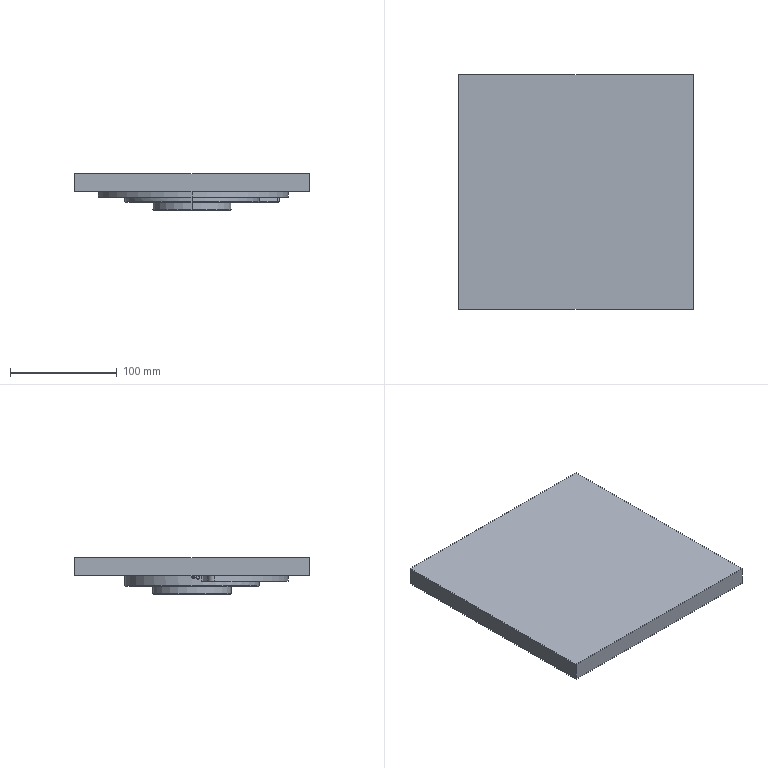NC program | NX | posted with a generic post | part box 220 x 220 x 34.5 mm
Lines 75 to 964 of 14163:
(ADAPTIVE_MILLING , TOOL : D10)
N118 T03 M6
N120 G54
N122 G17 G0 G90 X95.263 Y20.832 S8000 M3
N124 G43 Z30. H3
N126 Z-14.
N128 G94 G1 Z-17. F1000.
N130 X93.186 Y20.519 F3500.
N132 G3 X92.826 Y20.05 R0.517
N134 X93.039 Y13.768 R32.792
N136 G2 X93.561 Y-8.186 R106.889
N138 X-81.594 Y-46.533 R93.929
N140 X-84.05 Y-44.249 R11.158
N142 G3 X-84.843 Y-44.271 R0.524
N144 G1 X-86.022 Y-45.738
N146 G3 X-85.392 Y-46.489 R0.523
N148 G1 Z-14.
N150 G0 Z30.
N152 X95.262 Y18.312
N154 Z-14.
N156 G1 Z-17. F1000.
N158 G3 X94.965 Y19.276 R0.505 F3500.
N160 G1 X93.056 Y18.777
N162 G3 X92.762 Y18.381 R0.516
N164 X92.304 Y12.752 R16.402
N166 G2 X92.863 Y-0.982 R181.125
N168 X-79.677 Y-47.733 R92.885
N170 G1 X-79.748 Y-47.63
N172 X-79.823 Y-47.53
N174 X-79.915 Y-47.445
N176 X-79.934 Y-47.43
N178 G2 X-81.619 Y-46.513 R12.102
N180 G3 X-82.433 Y-46.766 R0.523
N182 G1 X-82.979 Y-48.467
N184 G3 X-82.283 Y-49.037 R0.523
N186 G1 Z-14.
N188 G0 Z30.
N190 X94.895 Y16.439
N192 Z-14.
N194 G1 Z-17. F1000.
N196 G3 X94.676 Y17.416 R0.505 F3500.
N198 G1 X92.8 Y17.246
N200 G3 X92.43 Y16.866 R0.513
N202 G2 X91.946 Y15.492 R15.396
N204 G3 X91.567 Y10.898 R17.162
N206 G2 X91.808 Y-1.348 R262.213
N208 X-77.715 Y-48.908 R91.827
N210 G3 X-78.616 Y-47.86 R3.744
N212 G2 X-80.011 Y-47.39 R8.929
N214 G3 X-80.769 Y-47.81 R0.523
N216 G1 X-80.913 Y-49.545
N218 G3 X-80.21 Y-49.992 R0.524
N220 G1 Z-14.
N222 G0 Z30.
N224 X94.546 Y15.319
N226 Z-14.
N228 G1 Z-17. F1000.
N230 G3 X94.362 Y16.297 R0.505 F3500.
N232 G1 X92.484 Y16.265
N234 G3 X92.109 Y15.965 R0.516
N236 X91.136 Y13.442 R15.341
N238 X90.756 Y7.716 R26.833
N240 G2 X90.504 Y-6.776 R155.471
N242 X-75.608 Y-50.206 R90.761
N244 G3 X-77.263 Y-48.18 R10.711
N246 X-78.032 Y-48.035 R2.623
N248 G1 X-78.631 Y-47.856
N250 G3 X-79.264 Y-48.21 R0.507
N252 G1 X-79.686 Y-49.83
N254 G3 X-79.007 Y-50.349 R0.506
N256 G1 Z-14.
N258 G0 Z30.
N260 X93.958 Y13.923
N262 Z-14.
N264 G1 Z-17. F1000.
N266 G3 X93.835 Y14.898 R0.505 F3500.
N268 G1 X92.028 Y15.079
N270 G3 X91.633 Y14.852 R0.518
N272 X90.105 Y10.683 R8.027
N274 X89.832 Y3.567 R65.162
N276 G2 X88.434 Y-14.983 R112.268
N278 X-73.656 Y-51.197 R89.698
N280 G3 X-75.959 Y-48.409 R15.928
N282 G1 X-76.056 Y-48.33
N284 X-76.166 Y-48.271
N286 X-76.268 Y-48.235
N288 X-77.511 Y-48.098
N290 G3 X-78.066 Y-48.524 R0.508
N292 G1 X-78.302 Y-50.139
N294 G3 X-77.621 Y-50.6 R0.507
N296 G1 Z-14.
N298 G0 Z30.
N300 X93.308 Y12.854
N302 Z-14.
N304 G1 Z-17. F1000.
N306 G3 X93.256 Y13.817 R0.505 F3500.
N308 G1 X91.553 Y14.242
N310 G3 X91.084 Y14.017 R0.514
N312 X89.98 Y12.255 R12.393
N314 X89.057 Y7.489 R15.658
N316 X88.653 Y-3.128 R811.962
N318 G2 X75.961 Y-45.688 R90.347
N320 X-71.996 Y-51.723 R88.653
N322 G3 X-74.658 Y-48.583 R20.077
N324 X-75.372 Y-48.187 R1.593
N326 G1 X-76.178 Y-48.244
N328 X-76.199 Y-48.243
N330 X-76.323 Y-48.229
N332 G3 X-76.883 Y-48.758 R0.507
N334 G1 X-76.787 Y-50.381
N336 G3 X-76.119 Y-50.742 R0.507
N338 G1 Z-14.
N340 G0 Z30.
N342 X92.742 Y11.989
N344 Z-14.
N346 G1 Z-17. F1000.
N348 G3 X92.721 Y12.943 R0.505 F3500.
N350 G1 X91.063 Y13.472
N352 G3 X90.621 Y13.321 R0.517
N354 X88.67 Y9.768 R6.422
N356 X87.922 Y2.819 R38.362
N358 G2 X86.66 Y-12.747 R143.741
N360 X-70.301 Y-52.254 R87.599
N362 G3 X-73.408 Y-48.671 R25.294
N364 X-74.378 Y-48.116 R1.953
N366 G1 X-75.376 Y-48.187
N368 G3 X-75.841 Y-48.757 R0.507
N370 G1 X-75.625 Y-50.335
N372 G3 X-74.967 Y-50.662 R0.507
N374 G1 Z-14.
N376 G0 Z30.
N378 X91.91 Y11.055
N380 Z-14.
N382 G1 Z-17. F1000.
N384 G3 X91.961 Y11.98 R0.506 F3500.
N386 G1 X90.448 Y12.731
N388 G3 X89.93 Y12.598 R0.513
N390 X87.822 Y8.894 R6.815
N392 X86.952 Y2.085 R37.463
N394 G2 X85.584 Y-12.847 R159.087
N396 X-68.777 Y-52.53 R86.556
N398 G3 X-72.272 Y-48.624 R27.922
N400 X-73.574 Y-47.926 R2.551
N402 G1 X-73.626 Y-47.927
N404 X-74.328 Y-48.108
N406 X-74.378 Y-48.116
N408 G3 X-74.799 Y-48.554 R0.51
N410 G1 X-74.987 Y-50.164
N412 G3 X-74.308 Y-50.613 R0.507
N414 G1 Z-14.
N416 G0 Z30.
N418 X91.197 Y10.305
N420 Z-14.
N422 G1 Z-17. F1000.
N424 G3 X91.278 Y11.214 R0.506 F3500.
N426 G1 X89.828 Y12.06
N428 G3 X89.35 Y11.998 R0.516
N430 X87.359 Y9.351 R5.041
N432 X86.138 Y3.241 R23.84
N434 G2 X85.011 Y-9.333 R410.242
N436 X45.334 Y-72.454 R85.909
N438 X-66.749 Y-53.391 R85.485
N440 G3 X-70.816 Y-48.82 R43.169
N442 X-72.606 Y-47.708 R5.013
N444 X-73.731 Y-47.954 R5.305
N446 X-74.089 Y-48.589 R0.507
N448 G1 X-73.628 Y-50.094
N450 G3 X-73. Y-50.346 R0.508
N452 G1 Z-14.
N454 G0 Z30.
N456 X90.606 Y9.825
N458 Z-14.
N460 G1 Z-17. F1000.
N462 G3 X90.725 Y10.709 R0.506 F3500.
N464 G1 X89.367 Y11.673
N466 G3 X88.844 Y11.631 R0.514
N468 X86.443 Y8.534 R5.723
N470 X85.149 Y2.309 R25.876
N472 G2 X83.848 Y-10.248 R397.442
N474 X52.239 Y-66.303 R85.08
N476 X-65.318 Y-53.487 R84.442
N478 G3 X-69.701 Y-48.696 R46.689
N480 X-71.827 Y-47.422 R5.598
N482 X-72.6 Y-47.663 R1.602
N484 G1 X-72.842 Y-47.725
N486 G3 X-73.221 Y-48.235 R0.509
N488 G1 X-73.148 Y-49.842
N490 G3 X-72.48 Y-50.21 R0.507
N492 G1 Z-14.
N494 G0 Z30.
N496 X89.732 Y9.188
N498 Z-14.
N500 G1 Z-17. F1000.
N502 G3 X89.902 Y10.033 R0.506 F3500.
N504 G1 X88.708 Y11.132
N506 G3 X88.136 Y11.117 R0.512
N508 X86.875 Y10.174 R6.334
N510 X84.987 Y6.131 R10.022
N512 X83.881 Y-0.901 R48.707
N514 G2 X81.827 Y-16.005 R155.534
N516 X-63.741 Y-53.73 R83.394
N518 G3 X-68.416 Y-48.695 R58.16
N520 X-71.069 Y-47.104 R6.574
N522 G1 X-71.193 Y-47.088
N524 X-71.318 Y-47.097
N526 X-71.404 Y-47.115
N528 X-72.199 Y-47.482
N530 G3 X-72.45 Y-48.141 R0.508
N532 G1 X-71.819 Y-49.585
N534 G3 X-71.222 Y-49.785 R0.509
N536 G1 Z-14.
N538 G0 Z30.
N540 X89.289 Y8.877
N542 Z-14.
N544 G1 Z-17. F1000.
N546 G3 X89.459 Y9.721 R0.506 F3500.
N548 G1 X88.243 Y10.838
N550 G3 X87.749 Y10.871 R0.515
N552 X85.183 Y8.436 R4.749
N554 X83.411 Y2.471 R19.563
N556 X81.986 Y-8.688 R517.85
N558 G2 X73.873 Y-36.265 R88.371
N560 X-61.814 Y-54.34 R82.311
N562 G3 X-67.114 Y-48.69 R77.33
N564 X-70.161 Y-46.784 R8.185
N566 X-70.921 Y-46.892 R0.817
N568 G1 X-71.489 Y-47.154
N570 G3 X-71.723 Y-47.848 R0.507
N572 G1 X-70.983 Y-49.237
N574 G3 X-70.407 Y-49.407 R0.51
N576 G1 Z-14.
N578 G0 Z30.
N580 X88.505 Y8.464
N582 Z-14.
N584 G1 Z-17. F1000.
N586 G3 X88.707 Y9.278 R0.507 F3500.
N588 G1 X87.607 Y10.485
N590 G3 X87.073 Y10.547 R0.514
N592 X84.312 Y7.961 R5.107
N594 X82.44 Y1.895 R20.41
N596 X80.859 Y-9.369 R520.037
N598 G2 X72.68 Y-36.28 R87.501
N600 X-60.52 Y-54.206 R81.258
N602 G3 X-65.97 Y-48.526 R86.986
N604 X-69.214 Y-46.456 R9.681
N606 X-70.054 Y-46.393 R1.418
N608 G1 X-70.812 Y-46.83
N610 G3 X-70.998 Y-47.518 R0.507
N612 G1 X-70.211 Y-48.883
N614 G3 X-69.645 Y-49.043 R0.51
N616 G1 Z-14.
N618 G0 Z30.
N620 X87.574 Y8.016
N622 Z-14.
N624 G1 Z-17. F1000.
N626 G3 X87.808 Y8.79 R0.507 F3500.
N628 G1 X86.85 Y10.079
N630 G3 X86.283 Y10.169 R0.512
N632 X83.984 Y8.415 R4.01
N634 X81.837 Y3.117 R15.49
N636 X80.458 Y-5.141 R96.52
N638 G2 X77.595 Y-20.237 R127.01
N640 X-58.819 Y-54.492 R80.201
N642 G3 X-64.753 Y-48.41 R109.578
N644 X-68.412 Y-46.067 R11.024
N646 X-69.343 Y-45.982 R1.646
N648 G1 X-70.101 Y-46.419
N650 G3 X-70.271 Y-47.132 R0.507
N652 G1 X-69.402 Y-48.456
N654 G3 X-68.858 Y-48.589 R0.512
N656 G1 Z-14.
N658 G0 Z30.
N660 X87.228 Y7.861
N662 Z-14.
N664 G1 Z-17. F1000.
N666 G3 X87.458 Y8.652 R0.511 F3500.
N668 G1 X86.442 Y9.954
N670 G3 X85.963 Y10.071 R0.52
N672 X83.165 Y8.134 R4.306
N674 X80.937 Y2.869 R15.704
N676 X79.288 Y-6.356 R99.899
N678 G2 X76.072 Y-21.762 R117.213
N680 X-57.365 Y-54.5 R79.15
N682 G3 X-63.618 Y-48.206 R124.294
N684 X-67.595 Y-45.666 R12.098
N686 X-68.612 Y-45.56 R1.821
N688 G1 X-69.37 Y-45.997
N690 G3 X-69.601 Y-46.586 R0.512
N692 G1 X-69.12 Y-48.126
N694 G3 X-68.493 Y-48.378 R0.511
N696 G1 Z-14.
N698 G0 Z30.
N700 X86.404 Y7.604
N702 Z-14.
N704 G1 Z-17. F1000.
N706 G3 X86.657 Y8.365 R0.512 F3500.
N708 G1 X85.75 Y9.727
N710 G3 X85.24 Y9.875 R0.519
N712 X82.332 Y7.875 R4.524
N714 X79.964 Y2.399 R16.403
N716 X78.26 Y-6.562 R100.821
N718 G2 X74.849 Y-22.181 R121.088
N720 X-55.352 Y-55.037 R78.08
N722 G3 X-61.9 Y-48.506 R282.175
N724 X-66.395 Y-45.385 R15.972
N726 X-67.727 Y-45.089 R3.8
N728 X-68.62 Y-45.565 R7.396
N730 X-68.844 Y-46.17 R0.51
N732 G1 X-68.305 Y-47.679
N734 G3 X-67.69 Y-47.914 R0.509
N736 G1 Z-14.
N738 G0 Z30.
N740 X85.573 Y7.376
N742 Z-14.
N744 G1 Z-17. F1000.
N746 G3 X85.843 Y8.101 R0.509 F3500.
N748 G1 X85.043 Y9.507
N750 G3 X84.516 Y9.678 R0.514
N752 X81.842 Y8.078 R4.093
N754 X79.283 Y2.971 R14.546
N756 X77.504 Y-5.207 R68.812
N758 G2 X74.552 Y-19.397 R156.429
N760 X13.634 Y-75.769 R77.294
N762 X-54.33 Y-54.564 R77.16
N764 G3 X-61.042 Y-48.02 R224.393
N766 X-65.691 Y-44.907 R16.072
N768 X-67.094 Y-44.684 R2.373
N770 G1 X-67.96 Y-45.184
N772 G3 X-68.177 Y-45.807 R0.509
N774 G1 X-67.58 Y-47.292
N776 G3 X-66.978 Y-47.503 R0.509
N778 G1 Z-14.
N780 G0 Z30.
N782 X84.578 Y7.146
N784 Z-14.
N786 G1 Z-17. F1000.
N788 G3 X84.905 Y7.703 R0.509 F3500.
N790 G1 X84.643 Y9.257
N792 G3 X84.076 Y9.595 R0.509
N794 X80.921 Y7.779 R4.453
N796 X78.269 Y2.438 R15.637
N798 X76.476 Y-5.482 R71.4
N800 G2 X73.189 Y-20.366 R151.28
N802 X10.738 Y-75.157 R76.194
N804 X-52.971 Y-54.419 R76.215
N806 G3 X-60.108 Y-47.596 R230.935
N808 X-64.774 Y-44.5 R17.094
N810 X-66.229 Y-44.207 R3.331
N812 G1 X-66.314 Y-44.233
N814 X-67.18 Y-44.733
N816 G3 X-67.393 Y-45.366 R0.509
N818 G1 X-66.769 Y-46.834
N820 G3 X-66.172 Y-47.038 R0.509
N822 G1 Z-14.
N824 G0 Z30.
N826 X84.266 Y7.092
N828 Z-14.
N830 G1 Z-17. F1000.
N832 G3 X84.553 Y7.792 R0.512 F3500.
N834 G1 X83.844 Y9.255
N836 G3 X83.338 Y9.465 R0.518
N838 X80.155 Y7.685 R4.596
N840 X77.44 Y2.516 R15.401
N842 X75.326 Y-6.354 R72.522
N844 G2 X72.025 Y-20.595 R149.329
N846 X18.659 Y-72.491 R75.245
N848 X-51.585 Y-54.267 R74.999
N850 G3 X-58.685 Y-47.587 R483.163
N852 X-63.719 Y-44.139 R20.181
N854 X-65.406 Y-43.741 R4.123
N856 G1 X-65.524 Y-43.777
N858 X-66.39 Y-44.277
N860 G3 X-66.6 Y-44.916 R0.509
N862 G1 X-65.957 Y-46.372
N864 G3 X-65.363 Y-46.571 R0.509
N866 G1 Z-14.
N868 G0 Z30.
N870 X83.451 Y6.948
N872 Z-14.
N874 G1 Z-17. F1000.
N876 G3 X83.747 Y7.621 R0.509 F3500.
N878 G1 X83.115 Y9.108
N880 G3 X82.599 Y9.335 R0.514
N882 X79.385 Y7.604 R4.662
N884 X76.491 Y2.251 R15.59
N886 X74.416 Y-5.985 R68.537
N888 G2 X71.042 Y-20.21 R163.02
N890 X36.627 Y-64.048 R74.504
N892 X-50.184 Y-54.12 R73.863
N894 G3 X-58.003 Y-46.927 R389.78
N896 X-62.994 Y-43.64 R19.61
N898 X-64.565 Y-43.271 R4.602
N900 X-65.582 Y-43.811 R5.383
N902 X-65.791 Y-44.453 R0.508
N904 G1 X-65.14 Y-45.903
N906 G3 X-64.548 Y-46.1 R0.509
N908 G1 Z-14.
N910 G0 Z30.
N912 X82.525 Y6.784
N914 Z-14.
N916 G1 Z-17. F1000.
N918 G3 X82.827 Y7.435 R0.507 F3500.
N920 G1 X82.266 Y8.932
N922 G3 X81.737 Y9.183 R0.51
N924 X78.525 Y7.44 R4.784
N926 X75.536 Y1.997 R16.094
N928 X73.303 Y-6.586 R71.811
N930 G2 X69.846 Y-20.534 R165.426
N932 X32.607 Y-64.999 R73.458
N934 X-48.864 Y-53.887 R72.821
N936 G3 X-56.645 Y-46.837 R656.247
N938 X-61.907 Y-43.277 R22.589
N940 X-63.831 Y-42.819 R4.013
N942 G1 X-63.906 Y-42.843
N944 X-64.772 Y-43.343
N946 G3 X-64.981 Y-43.985 R0.508
N948 G1 X-64.329 Y-45.435
N950 G3 X-63.737 Y-45.632 R0.509
N952 G1 Z-14.
N954 G0 Z30.
N956 X81.732 Y6.644
N958 Z-14.
N960 G1 Z-17. F1000.
N962 G3 X82.04 Y7.278 R0.508 F3500.
N964 G1 X81.535 Y8.788
N966 G3 X80.999 Y9.053 R0.51
N968 X77.577 Y7.192 R5.01
N970 X74.49 Y1.518 R16.93
N972 X72.348 Y-6.444 R73.694
N974 G2 X68.684 Y-20.726 R167.44
N976 X40.916 Y-58.808 R72.658
N978 X-47.623 Y-53.567 R71.72
N980 G3 X-55.846 Y-46.262 R645.36
N982 X-61.152 Y-42.769 R22.594
N984 X-62.96 Y-42.333 R4.677
N986 X-63.953 Y-42.87 R13.452
N988 X-64.163 Y-43.512 R0.508
N990 G1 X-63.511 Y-44.963
N992 G3 X-62.919 Y-45.16 R0.509
N994 G1 Z-14.
N996 G0 Z30.
N998 X80.845 Y6.488
N1000 Z-14.
N1002 G1 Z-17. F1000.
N1004 G3 X81.156 Y7.114 R0.508 F3500.
N1006 G1 X80.677 Y8.629
N1008 G3 X80.137 Y8.901 R0.51
N1010 X76.708 Y7.049 R5.052
N1012 X73.608 Y1.522 R16.9
N1014 X71.251 Y-6.899 R75.673
N1016 G2 X67.6 Y-20.668 R170.674
N1018 X43.838 Y-55.304 R72.013
N1020 X-46.177 Y-53.41 R70.627
N1022 G1 X-46.654 Y-53.006
N1024 X-47.129 Y-52.599
N1026 X-47.695 Y-52.107
N1028 X-48.259 Y-51.613
N1030 X-48.915 Y-51.033
N1032 X-49.755 Y-50.286
N1034 X-51.154 Y-49.037
N1036 X-51.623 Y-48.624
N1038 X-51.716 Y-48.54
N1040 X-52.468 Y-47.881
N1042 X-53.128 Y-47.306
N1044 X-53.696 Y-46.816
N1046 X-54.172 Y-46.412
N1048 G3 X-59.811 Y-42.51 R28.138
N1050 X-62.074 Y-41.847 R6.008
N1052 X-63.121 Y-42.39 R4.046
N1054 X-63.328 Y-43.039 R0.508
N1056 G1 X-62.656 Y-44.477
N1058 G3 X-62.068 Y-44.668 R0.51
N1060 G1 Z-14.
N1062 G0 Z30.
N1064 X79.963 Y6.332
N1066 Z-14.
N1068 G1 Z-17. F1000.
N1070 G3 X80.276 Y6.951 R0.508 F3500.
N1072 G1 X79.817 Y8.472
N1074 G3 X79.275 Y8.749 R0.51
N1076 X75.836 Y6.912 R5.107
N1078 X72.684 Y1.414 R17.091
N1080 X69.97 Y-8.074 R82.76
N1082 G2 X65.822 Y-22.611 R142.782
N1084 X24.526 Y-65.04 R70.234
N1086 X-45.296 Y-52.769 R69.705
N1088 G3 X-53.836 Y-45.446 R875.946
N1090 X-59.373 Y-41.846 R24.637
N1092 X-61.299 Y-41.374 R4.902
N1094 X-62.293 Y-41.912 R13.853
N1096 X-62.472 Y-42.61 R0.507
N1098 G1 X-61.645 Y-43.962
N1100 G3 X-61.094 Y-44.106 R0.512
N1102 G1 Z-14.
N1104 G0 Z30.
N1106 X79.093 Y6.179
N1108 Z-14.
N1110 G1 Z-17. F1000.
N1112 G3 X79.407 Y6.796 R0.508 F3500.
N1114 G1 X78.957 Y8.317
N1116 G3 X78.414 Y8.597 R0.51
N1118 X74.875 Y6.69 R5.247
N1120 X71.575 Y0.847 R18.131
N1122 X68.856 Y-8.511 R90.852
N1124 G2 X64.899 Y-22.064 R146.408
N1126 X33.453 Y-59.699 R69.521
N1128 X-43.441 Y-52.918 R68.529
N1130 X-52.04 Y-45.665 R812.015
N1132 G3 X-58.126 Y-41.533 R30.286
N1134 X-60.393 Y-40.881 R6.308
N1136 X-61.45 Y-41.425 R3.873
N1138 X-61.636 Y-42.112 R0.507
N1140 G1 X-60.849 Y-43.478
N1142 G3 X-60.284 Y-43.638 R0.51
N1144 G1 Z-14.
N1146 G0 Z30.
N1148 X78.231 Y6.027
N1150 Z-14.
N1152 G1 Z-17. F1000.
N1154 G3 X78.546 Y6.644 R0.508 F3500.
N1156 G1 X78.095 Y8.166
N1158 G3 X77.552 Y8.445 R0.51
N1160 X73.998 Y6.563 R5.279
N1162 X70.73 Y0.986 R17.845
N1164 X68.053 Y-7.731 R77.89
N1166 X66.647 Y-14.231 R45.706
N1168 G1 X65.388 Y-19.203
N1170 X65.382 Y-19.223
N1172 X63.751 Y-24.086
N1174 X63.744 Y-24.106
N1176 X61.75 Y-28.832
N1178 X61.741 Y-28.851
N1180 X59.397 Y-33.413
N1182 X59.386 Y-33.431
N1184 X56.704 Y-37.803
N1186 X56.692 Y-37.82
N1188 X53.687 Y-41.977
N1190 X53.674 Y-41.994
N1192 X50.364 Y-45.911
N1194 X50.35 Y-45.927
N1196 X46.753 Y-49.584
N1198 X46.737 Y-49.598
N1200 X42.875 Y-52.973
N1202 X42.858 Y-52.986
N1204 X38.752 Y-56.059
N1206 X38.735 Y-56.071
N1208 X34.408 Y-58.826
N1210 X34.39 Y-58.836
N1212 X29.867 Y-61.256
N1214 X29.848 Y-61.265
N1216 X25.156 Y-63.337
N1218 X25.136 Y-63.345
N1220 X20.301 Y-65.056
N1222 X20.281 Y-65.062
N1224 X15.33 Y-66.403
N1226 X15.31 Y-66.408
N1228 X10.272 Y-67.371
N1230 X10.251 Y-67.374
N1232 X5.155 Y-67.954
N1234 X5.134 Y-67.956
N1236 X-0.002 Y-68.15
N1238 X-5.045 Y-67.963
N1240 X-5.065 Y-67.961
N1242 X-10.07 Y-67.402
N1244 X-10.091 Y-67.398
N1246 X-15.04 Y-66.469
N1248 X-15.06 Y-66.465
N1250 X-19.927 Y-65.171
N1252 X-19.947 Y-65.165
N1254 X-24.704 Y-63.514
N1256 X-24.724 Y-63.507
N1258 X-29.345 Y-61.508
N1260 X-29.364 Y-61.499
N1262 X-33.825 Y-59.163
N1264 X-33.843 Y-59.152
N1266 X-38.119 Y-56.492
N1268 X-38.136 Y-56.48
N1270 X-42.203 Y-53.51
N1272 X-42.219 Y-53.497
N1274 X-46.054 Y-50.234
N1276 X-46.069 Y-50.219
N1278 G3 X-51.585 Y-44.906 R121.246
N1280 X-57.6 Y-40.904 R25.156
N1282 X-59.646 Y-40.409 R4.744
N1284 G1 X-59.742 Y-40.439
N1286 X-60.608 Y-40.939
N1288 G3 X-60.654 Y-41.862 R0.551
N1290 G1 X-58.903 Y-42.828 Z-16.9
N1292 X-53.981 Y-45.529
N1294 X-52.228 Y-46.491 Z-17.
N1296 X-50.234 Y-47.577
N1298 G3 X-49.652 Y-46.681 R0.55
N1300 X-53.006 Y-42.948 R57.94
N1302 X-58.034 Y-40.01 R12.724
N1304 X-58.917 Y-39.962 R1.787
N1306 G1 X-59.783 Y-40.462
N1308 G3 X-59.735 Y-41.44 R0.551
N1310 G1 X-52.854 Y-44.543
N1312 G3 X-52.295 Y-43.651 R0.55
N1314 G1 X-54.004 Y-41.587
N1316 G3 X-57.895 Y-39.484 R6.966
N1318 G1 X-58.02 Y-39.491
N1320 X-58.141 Y-39.522
N1322 X-58.169 Y-39.53
N1324 X-58.926 Y-39.968
N1326 G3 X-58.864 Y-40.951 R0.551
N1328 G1 X-54.157 Y-42.919
N1330 G3 X-53.589 Y-42.054 R0.551
N1332 X-55.273 Y-40.052 R10.623
N1334 X-57.415 Y-39.135 R3.59
N1336 X-58.198 Y-39.548 R7.813
N1338 X-58.111 Y-40.541 R0.551
N1340 G1 X-55.106 Y-41.624
N1342 G3 X-54.563 Y-40.754 R0.551
N1344 X-55.983 Y-39.194 R5.616
N1346 X-57.103 Y-38.915 R1.383
N1348 G1 X-57.645 Y-39.228
N1350 G3 X-57.52 Y-40.233 R0.551
N1352 G1 X-55.739 Y-40.73
N1354 G3 X-55.238 Y-39.853 R0.551
N1356 X-56.271 Y-38.792 R3.011
N1358 X-57.158 Y-38.947 R0.848
N1360 X-56.997 Y-39.961 R0.551
N1362 G1 X-56.154 Y-40.132
N1364 G3 X-55.688 Y-39.253 R0.551
N1366 X-56.449 Y-38.64 R1.105
N1368 X-56.876 Y-38.784 R4.335
N1370 X-56.434 Y-39.784 R0.55
N1372 X-55.982 Y-39.527 R0.772
N1374 X-56.248 Y-38.682 R0.555
N1376 X-56.733 Y-40.493 R1.123
N1378 G1 Z-14.
N1380 G0 Z30.
N1382 X77.175 Y6.482
N1384 Z-14.
N1386 G1 Z-17. F1000.
N1388 G3 X76.69 Y8.293 R0.946 F3500.
N1390 X73.117 Y6.445 R5.308
N1392 X69.794 Y0.901 R17.916
N1394 X67.997 Y-4.374 R60.179
N1396 G1 X67.534 Y-9.136
N1398 X67.532 Y-9.157
N1400 X67.253 Y-10.758
N1402 G3 X68.299 Y-11.072 R0.55
N1404 G1 X69.501 Y-8.305
N1406 X70.298 Y-6.471 Z-16.9
N1408 X75.51 Y5.528
N1410 X76.307 Y7.362 Z-17.
N1412 G3 X75.705 Y8.119 R0.551
N1414 X72.236 Y6.325 R5.313
N1416 X68.805 Y0.702 R17.969
N1418 G1 X68.71 Y0.471
N1420 X68.569 Y0.123
N1422 X68.433 Y-0.226
N1424 X68.3 Y-0.577
N1426 X68.127 Y-1.046
N1428 X68.092 Y-1.176
N1430 X67.994 Y-4.404
N1432 G3 X69.026 Y-4.718 R0.55
N1434 G1 X69.621 Y-3.613
N1436 X70.569 Y-1.852 Z-16.9
N1438 X74.443 Y5.344
N1440 X75.391 Y7.105 Z-17.
N1442 G3 X74.844 Y7.967 R0.554
N1444 X71.264 Y6.125 R5.422
N1446 X68.138 Y1.176 R16.417
N1448 G1 X68.141 Y1.124
N1450 X68.09 Y-1.25
N1452 G3 X69.107 Y-1.553 R0.55
N1454 G1 X69.568 Y-0.814
N1456 X70.627 Y0.883 Z-16.9
N1458 X73.286 Y5.142
N1460 X74.345 Y6.839 Z-17.
N1462 G3 X74.454 Y7.481 R0.635
N1464 X73.859 Y7.794 R0.555
N1466 X70.289 Y5.93 R5.471
N1468 X68.071 Y2.774 R12.189
N1470 G1 X68.056 Y2.686
N1472 X68.14 Y1.136
N1474 G3 X69.131 Y0.838 R0.551
N1476 G1 X73.581 Y6.847
N1478 G3 X72.997 Y7.642 R0.551
N1480 X69.311 Y5.739 R5.582
N1482 X67.998 Y3.933 R5.395
N1484 G1 X67.991 Y3.888
N1486 X68.058 Y2.639
N1488 G3 X69.032 Y2.32 R0.551
N1490 G1 X72.583 Y6.651
N1492 G3 X72.012 Y7.468 R0.551
N1494 X67.997 Y5.016 R5.307
N1496 X67.995 Y3.801 R3.527
N1498 X68.95 Y3.459 R0.551
N1500 G1 X71.707 Y6.475
N1502 G3 X71.151 Y7.316 R0.551
N1504 X68.701 Y6.469 R5.106
N1506 X67.904 Y5.47 R1.79
N1508 G1 X67.945 Y4.721
N1510 G3 X68.892 Y4.371 R0.551
N1512 G1 X70.713 Y6.288
N1514 G3 X70.166 Y7.143 R0.551
N1516 X68.389 Y6.605 R4.194
N1518 X67.907 Y5.414 R1.055
N1520 X68.858 Y5.068 R0.551
N1522 G1 X69.854 Y6.14
N1524 G3 X69.304 Y6.991 R0.551
N1526 X68.029 Y6.549 R2.244
N1528 X67.886 Y5.8 R0.944
N1530 X68.89 Y5.52 R0.55
N1532 G1 X69.281 Y6.105
N1534 G3 X68.689 Y6.882 R0.551
N1536 X67.887 Y6.362 R0.803
N1538 G1 X67.865 Y6.207
N1540 X67.866 Y6.176
N1542 X67.873 Y6.051
N1544 G3 X68.229 Y5.537 R0.606
N1546 G1 X70.458 Y4.557
N1548 Z-14.
N1550 G0 Z30.
N1552 X43.546 Y-2.752
N1554 Z3.
N1556 G3 X43.546 Y-2.752 Z2.506 I4.392 J-0.978 F1000.
N1558 X43.546 Y-2.752 Z2.013 I4.392 J-0.978
N1560 X43.546 Y-2.752 Z1.519 I4.392 J-0.978
N1562 X43.546 Y-2.752 Z1.026 I4.392 J-0.978
N1564 X43.546 Y-2.752 Z0.532 I4.392 J-0.978
N1566 X43.546 Y-2.752 Z0.039 I4.392 J-0.978
N1568 X43.546 Y-2.752 Z-0.455 I4.392 J-0.978
N1570 X43.546 Y-2.752 Z-0.948 I4.392 J-0.978
N1572 X43.546 Y-2.752 Z-1.442 I4.392 J-0.978
N1574 X43.546 Y-2.752 Z-1.935 I4.392 J-0.978
N1576 X43.546 Y-2.752 Z-2.429 I4.392 J-0.978
N1578 X43.546 Y-2.752 Z-2.922 I4.392 J-0.978
N1580 X43.546 Y-2.752 Z-3.416 I4.392 J-0.978
N1582 X43.546 Y-2.752 Z-3.909 I4.392 J-0.978
N1584 X43.546 Y-2.752 Z-4.403 I4.392 J-0.978
N1586 X43.546 Y-2.752 Z-4.896 I4.392 J-0.978
N1588 X43.546 Y-2.752 Z-5.39 I4.392 J-0.978
N1590 X43.546 Y-2.752 Z-5.884 I4.392 J-0.978
N1592 X43.546 Y-2.752 Z-6.377 I4.392 J-0.978
N1594 X43.546 Y-2.752 Z-6.871 I4.392 J-0.978
N1596 X43.546 Y-2.752 Z-7.364 I4.392 J-0.978
N1598 X43.546 Y-2.752 Z-7.858 I4.392 J-0.978
N1600 X43.546 Y-2.752 Z-8.351 I4.392 J-0.978
N1602 X43.546 Y-2.752 Z-8.845 I4.392 J-0.978
N1604 X43.546 Y-2.752 Z-9.338 I4.392 J-0.978
N1606 X43.546 Y-2.752 Z-9.832 I4.392 J-0.978
N1608 X43.438 Y-3.73 Z-9.849 R4.5
N1610 X44.26 Y-1.125 R-4.501 F3500.
N1612 X48.93 Y-8.598 R4.669
N1614 X44.132 Y-0.487 R-4.978
N1616 X49.902 Y-8.823 R5.193
N1618 X44.254 Y0.351 R-5.475
N1620 X50.347 Y-9.199 R5.719
N1622 X44.414 Y1.147 R-5.995
N1624 X50.878 Y-9.543 R6.258
N1626 X44.273 Y1.716 R-6.538
N1628 X50.829 Y-10.18 R6.809
N1630 X44.4 Y2.452 R-7.095
N1632 X41.033 Y-1.504 R7.259
N1634 X50.368 Y-11.012 R7.378
N1636 X54.85 Y-7.089 R7.551
N1638 X55.229 Y-2.087 R31.46
N1640 X50.718 Y3.452 R6.947
N1642 X40.594 Y-0.915 R7.895
N1644 G2 X40.303 Y-5.147 R35.23
N1646 G3 X43.296 Y-10.515 R6.815
N1648 X54.637 Y-8.653 R8.175
N1650 X54.856 Y-7.038 R16.536
N1652 G1 X55.247 Y-2.586
N1654 G3 X55.128 Y-0.228 R7.165
N1656 X50.395 Y4.227 R7.101
N1658 X40.692 Y0.647 R8.491
N1660 X40.591 Y-1.005 R9.172
N1662 X41.06 Y-1.57 R0.554
N1664 G1 X43.059 Y-1.617 Z-9.749
N1666 X52.665 Y-1.824
N1668 X54.664 Y-1.867 Z-9.849
N1670 G3 X55.288 Y-1.337 R0.558
N1672 X54.823 Y1.451 R4.783
N1674 X49.05 Y5.18 R7.673
N1676 X40.753 Y1.819 R8.932
N1678 X40.59 Y1.421 R2.824
N1680 G1 X40.647 Y0.494
N1682 G3 X41.119 Y-0.034 R0.554
N1684 G1 X43.115 Y-0.158 Z-9.749
N1686 X52.658 Y-0.741
N1688 X54.654 Y-0.863 Z-9.849
N1690 G3 X55.321 Y-0.337 R0.563
N1692 X53.912 Y3.483 R4.482
N1694 X45.333 Y5.6 R8.862
N1696 X40.733 Y2.755 R8.586
N1698 X40.535 Y2.302 R1.351
N1700 G1 X40.597 Y1.304
N1702 G3 X41.133 Y0.788 R0.554
N1704 G1 X43.131 Y0.7 Z-9.749
N1706 X52.649 Y0.279
N1708 X54.647 Y0.19 Z-9.849
N1710 G3 X55.334 Y0.762 R0.573
N1712 X53.613 Y4.482 R4.565
N1714 X45.025 Y6.22 R9.279
N1716 X40.774 Y3.722 R8.645
N1718 X40.483 Y3.152 R1.395
N1720 G1 X40.537 Y2.279
N1722 G3 X41.074 Y1.763 R0.554
N1724 G1 X43.072 Y1.66 Z-9.749
N1726 X52.642 Y1.166
N1728 X54.639 Y1.063 Z-9.849
N1730 G3 X55.29 Y1.636 R0.558
N1732 X53.659 Y5.133 R4.313
N1734 X46.048 Y7.145 R9.338
N1736 X40.919 Y4.753 R9.284
N1738 X40.433 Y3.964 R1.637
N1740 G1 X40.487 Y3.091
N1742 G3 X41.025 Y2.575 R0.554
N1744 G1 X43.022 Y2.462 Z-9.749
N1746 X52.636 Y1.923
N1748 X54.633 Y1.811 Z-9.849
N1750 G3 X55.252 Y2.385 R0.554
N1752 X53.692 Y5.782 R4.174
N1754 X46.461 Y7.896 R9.431
N1756 X40.996 Y5.665 R9.593
N1758 X40.372 Y4.68 R1.602
N1760 G1 X40.397 Y4.524
N1762 X40.4 Y4.496
N1764 X40.438 Y3.872
N1766 G3 X40.977 Y3.356 R0.554
N1768 G1 X42.974 Y3.239 Z-9.749
N1770 X52.629 Y2.675
N1772 X54.626 Y2.558 Z-9.849
N1774 G3 X55.214 Y3.134 R0.552
N1776 X53.624 Y6.514 R4.141
N1778 X46.622 Y8.61 R9.564
N1780 X41.083 Y6.558 R9.788
N1782 X40.271 Y5.473 R2.489
N1784 G1 X40.263 Y5.348
N1786 X40.383 Y4.608
N1788 G3 X40.93 Y4.144 R0.556
N1790 G1 X42.927 Y4.022 Z-9.749
N1792 X52.625 Y3.427
N1794 X54.621 Y3.306 Z-9.849
N1796 G3 X55.177 Y3.883 R0.552
N1798 X53.645 Y7.159 R4.021
N1800 X47.031 Y9.333 R9.567
N1802 X41.082 Y7.359 R9.992
N1804 X40.166 Y6.195 R2.988
N1806 X40.27 Y5.304 R4.658
N1808 X40.884 Y4.837 R0.576
N1810 G1 X42.881 Y4.723 Z-9.749
N1812 X52.618 Y4.166
N1814 X54.615 Y4.055 Z-9.849
N1816 G3 X55.139 Y4.632 R0.553
N1818 X53.387 Y8.038 R4.216
N1820 X46.455 Y10.011 R9.958
N1822 X40.999 Y8.083 R9.728
N1824 X40.041 Y6.808 R2.446
N1826 G1 X40.037 Y6.744
N1828 X40.157 Y6.003
N1830 G3 X40.777 Y5.537 R0.577
N1832 G1 X42.775 Y5.438 Z-9.749
N1834 X52.603 Y4.95
N1836 X54.546 Y4.856 Z-9.846
N1838 X54.601 Y4.862 Z-9.849
N1840 G3 X55.063 Y5.479 R0.553
N1842 X53.186 Y8.851 R4.322
N1844 X45.964 Y10.686 R10.256
N1846 X40.696 Y8.62 R9.298
N1848 X39.928 Y7.508 R2.211
N1850 G1 X39.924 Y7.444
N1852 X40.044 Y6.704
N1854 G3 X40.658 Y6.239 R0.571
N1856 G1 X42.657 Y6.163 Z-9.749
N1858 X52.49 Y5.794
N1860 X54.435 Y5.724 Z-9.846
N1862 X54.488 Y5.73 Z-9.849
N1864 G3 X54.946 Y6.346 R0.553
N1866 X53.172 Y9.507 R4.175
N1868 X46.34 Y11.429 R10.136
N1870 X40.765 Y9.483 R9.713
N1872 X39.813 Y8.205 R2.405
N1874 G1 X39.81 Y8.148
N1876 X39.93 Y7.407
N1878 G3 X40.543 Y6.942 R0.569
N1880 G1 X42.541 Y6.873 Z-9.749
N1882 X52.391 Y6.532
N1884 X53.39 Y6.49 Z-9.799
N1886 X54.39 Y6.473 Z-9.849
N1888 G3 X54.847 Y7.089 R0.553
N1890 X53.153 Y10.16 R4.073